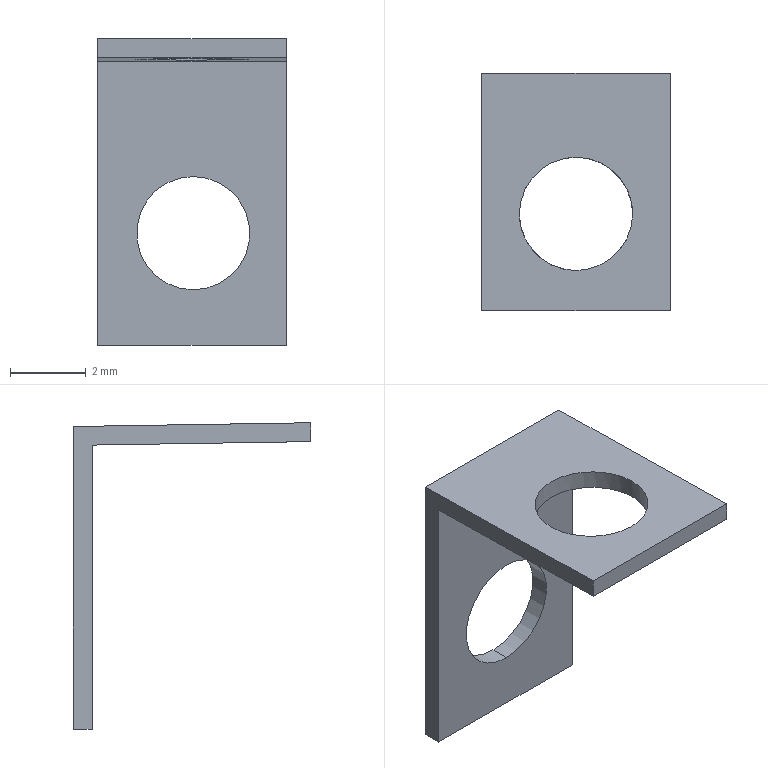Part | SolidWorks | features SplitBody 1 | 1 solid | 12 faces | box 5 x 6.285 x 8.118 mm | volume 27.45 mm3 | plane 8 | cylinder 4 | commonest cylinder face diameters 3 x4
STEP:
#1=CARTESIAN_POINT('',(-22.821,-45.477,-19.331));
#2=VERTEX_POINT('',#1);
#3=CARTESIAN_POINT('',(-19.821,-45.477,-19.331));
#4=VERTEX_POINT('',#3);
#5=CARTESIAN_POINT('',(-22.821,-45.477,-19.331));
#6=CARTESIAN_POINT('',(-22.821,-48.477,-19.284));
#7=CARTESIAN_POINT('',(-19.821,-48.477,-19.284));
#8=CARTESIAN_POINT('',(-19.821,-45.477,-19.331));
#9=(BOUNDED_CURVE()B_SPLINE_CURVE(3,(#5,#6,#7,#8),.UNSPECIFIED.,.F.,.F.)B_SPLINE_CURVE_WITH_KNOTS((4,4),(4.712,7.854),.UNSPECIFIED.)CURVE()GEOMETRIC_REPRESENTATION_ITEM()RATIONAL_B_SPLINE_CURVE((1.,0.3333,0.3333,1.))REPRESENTATION_ITEM(''));
#10=EDGE_CURVE('',#2,#4,#9,.T.);
#11=ORIENTED_EDGE('',*,*,#10,.F.);
#12=CARTESIAN_POINT('',(-22.821,-45.477,-18.831));
#13=VERTEX_POINT('',#12);
#14=CARTESIAN_POINT('',(-22.821,-45.477,-30.));
#15=DIRECTION('',(0.,0.,1.));
#16=VECTOR('',#15,1000.);
#17=LINE('',#14,#16);
#18=EDGE_CURVE('',#2,#13,#17,.T.);
#19=ORIENTED_EDGE('',*,*,#18,.T.);
#20=CARTESIAN_POINT('',(-19.821,-45.477,-18.831));
#21=VERTEX_POINT('',#20);
#22=CARTESIAN_POINT('',(-19.821,-45.477,-18.831));
#23=CARTESIAN_POINT('',(-19.821,-48.477,-18.784));
#24=CARTESIAN_POINT('',(-22.821,-48.477,-18.784));
#25=CARTESIAN_POINT('',(-22.821,-45.477,-18.831));
#26=(BOUNDED_CURVE()B_SPLINE_CURVE(3,(#22,#23,#24,#25),.UNSPECIFIED.,.F.,.F.)B_SPLINE_CURVE_WITH_KNOTS((4,4),(4.712,7.854),.UNSPECIFIED.)CURVE()GEOMETRIC_REPRESENTATION_ITEM()RATIONAL_B_SPLINE_CURVE((1.,0.3333,0.3333,1.))REPRESENTATION_ITEM(''));
#27=EDGE_CURVE('',#21,#13,#26,.T.);
#28=ORIENTED_EDGE('',*,*,#27,.F.);
#29=CARTESIAN_POINT('',(-19.821,-45.477,-30.));
#30=DIRECTION('',(0.,0.,1.));
#31=VECTOR('',#30,1000.);
#32=LINE('',#29,#31);
#33=EDGE_CURVE('',#4,#21,#32,.T.);
#34=ORIENTED_EDGE('',*,*,#33,.F.);
#35=EDGE_LOOP('',(#11,#19,#28,#34));
#36=FACE_OUTER_BOUND('',#35,.T.);
#37=CARTESIAN_POINT('',(-21.321,-45.477,-30.));
#38=DIRECTION('',(0.,0.,1.));
#39=DIRECTION('',(1.,0.,0.));
#40=AXIS2_PLACEMENT_3D('',#37,#38,#39);
#41=CYLINDRICAL_SURFACE('',#40,1.5);
#42=ADVANCED_FACE('',(#36),#41,.F.);
#43=CARTESIAN_POINT('',(-21.288,-41.756,-22.441));
#44=VERTEX_POINT('',#43);
#45=CARTESIAN_POINT('',(-21.288,-41.756,-25.441));
#46=VERTEX_POINT('',#45);
#47=CARTESIAN_POINT('',(-21.288,-41.756,-23.941));
#48=DIRECTION('',(0.,-1.,0.));
#49=DIRECTION('',(0.,0.,-1.));
#50=AXIS2_PLACEMENT_3D('',#47,#48,#49);
#51=CIRCLE('',#50,1.5);
#52=EDGE_CURVE('',#44,#46,#51,.T.);
#53=ORIENTED_EDGE('',*,*,#52,.F.);
#54=CARTESIAN_POINT('',(-21.288,-42.256,-22.441));
#55=VERTEX_POINT('',#54);
#56=CARTESIAN_POINT('',(-21.288,-37.256,-22.441));
#57=DIRECTION('',(0.,-1.,0.));
#58=VECTOR('',#57,1000.);
#59=LINE('',#56,#58);
#60=EDGE_CURVE('',#44,#55,#59,.T.);
#61=ORIENTED_EDGE('',*,*,#60,.T.);
#62=CARTESIAN_POINT('',(-21.288,-42.256,-25.441));
#63=VERTEX_POINT('',#62);
#64=CARTESIAN_POINT('',(-21.288,-42.256,-23.941));
#65=DIRECTION('',(0.,1.,0.));
#66=DIRECTION('',(0.,0.,1.));
#67=AXIS2_PLACEMENT_3D('',#64,#65,#66);
#68=CIRCLE('',#67,1.5);
#69=EDGE_CURVE('',#63,#55,#68,.T.);
#70=ORIENTED_EDGE('',*,*,#69,.F.);
#71=CARTESIAN_POINT('',(-21.288,-37.256,-25.441));
#72=DIRECTION('',(0.,-1.,0.));
#73=VECTOR('',#72,1000.);
#74=LINE('',#71,#73);
#75=EDGE_CURVE('',#46,#63,#74,.T.);
#76=ORIENTED_EDGE('',*,*,#75,.F.);
#77=EDGE_LOOP('',(#53,#61,#70,#76));
#78=FACE_OUTER_BOUND('',#77,.T.);
#79=CARTESIAN_POINT('',(-21.288,-37.256,-23.941));
#80=DIRECTION('',(0.,-1.,0.));
#81=DIRECTION('',(0.,0.,-1.));
#82=AXIS2_PLACEMENT_3D('',#79,#80,#81);
#83=CYLINDRICAL_SURFACE('',#82,1.5);
#84=ADVANCED_FACE('',(#78),#83,.F.);
#85=CARTESIAN_POINT('',(-23.821,-48.041,-18.791));
#86=VERTEX_POINT('',#85);
#87=CARTESIAN_POINT('',(-23.821,-48.041,-19.291));
#88=VERTEX_POINT('',#87);
#89=CARTESIAN_POINT('',(-23.821,-48.041,-18.791));
#90=DIRECTION('',(0.,0.,-1.));
#91=VECTOR('',#90,1000.);
#92=LINE('',#89,#91);
#93=EDGE_CURVE('',#86,#88,#92,.T.);
#94=ORIENTED_EDGE('',*,*,#93,.T.);
#95=CARTESIAN_POINT('',(-18.821,-48.041,-19.291));
#96=VERTEX_POINT('',#95);
#97=CARTESIAN_POINT('',(-18.821,-48.041,-19.291));
#98=DIRECTION('',(-1.,0.,0.));
#99=VECTOR('',#98,1000.);
#100=LINE('',#97,#99);
#101=EDGE_CURVE('',#96,#88,#100,.T.);
#102=ORIENTED_EDGE('',*,*,#101,.F.);
#103=CARTESIAN_POINT('',(-18.821,-48.041,-18.791));
#104=VERTEX_POINT('',#103);
#105=CARTESIAN_POINT('',(-18.821,-48.041,-18.791));
#106=DIRECTION('',(0.,0.,-1.));
#107=VECTOR('',#106,1000.);
#108=LINE('',#105,#107);
#109=EDGE_CURVE('',#104,#96,#108,.T.);
#110=ORIENTED_EDGE('',*,*,#109,.F.);
#111=CARTESIAN_POINT('',(-18.821,-48.041,-18.791));
#112=DIRECTION('',(-1.,0.,0.));
#113=VECTOR('',#112,1000.);
#114=LINE('',#111,#113);
#115=EDGE_CURVE('',#104,#86,#114,.T.);
#116=ORIENTED_EDGE('',*,*,#115,.T.);
#117=EDGE_LOOP('',(#94,#102,#110,#116));
#118=FACE_OUTER_BOUND('',#117,.T.);
#119=CARTESIAN_POINT('',(-18.821,-48.041,-18.791));
#120=DIRECTION('',(0.,1.,0.));
#121=DIRECTION('',(0.,0.,1.));
#122=AXIS2_PLACEMENT_3D('',#119,#120,#121);
#123=PLANE('',#122);
#124=ADVANCED_FACE('',(#118),#123,.F.);
#125=CARTESIAN_POINT('',(-19.821,-45.477,-19.331));
#126=CARTESIAN_POINT('',(-19.821,-42.477,-19.379));
#127=CARTESIAN_POINT('',(-22.821,-42.477,-19.379));
#128=CARTESIAN_POINT('',(-22.821,-45.477,-19.331));
#129=(BOUNDED_CURVE()B_SPLINE_CURVE(3,(#125,#126,#127,#128),.UNSPECIFIED.,.F.,.F.)B_SPLINE_CURVE_WITH_KNOTS((4,4),(1.571,4.712),.UNSPECIFIED.)CURVE()GEOMETRIC_REPRESENTATION_ITEM()RATIONAL_B_SPLINE_CURVE((1.,0.3333,0.3333,1.))REPRESENTATION_ITEM(''));
#130=EDGE_CURVE('',#4,#2,#129,.T.);
#131=ORIENTED_EDGE('',*,*,#130,.T.);
#132=ORIENTED_EDGE('',*,*,#10,.T.);
#133=EDGE_LOOP('',(#131,#132));
#134=FACE_BOUND('',#133,.T.);
#135=CARTESIAN_POINT('',(-23.821,-42.256,-19.382));
#136=VERTEX_POINT('',#135);
#137=CARTESIAN_POINT('',(-23.821,-48.041,-19.291));
#138=DIRECTION('',(0.,0.9999,-0.01579));
#139=VECTOR('',#138,1000.);
#140=LINE('',#137,#139);
#141=EDGE_CURVE('',#88,#136,#140,.T.);
#142=ORIENTED_EDGE('',*,*,#141,.T.);
#143=CARTESIAN_POINT('',(-18.821,-42.256,-19.382));
#144=VERTEX_POINT('',#143);
#145=CARTESIAN_POINT('',(-18.821,-42.256,-19.382));
#146=DIRECTION('',(-1.,0.,0.));
#147=VECTOR('',#146,1000.);
#148=LINE('',#145,#147);
#149=EDGE_CURVE('',#144,#136,#148,.T.);
#150=ORIENTED_EDGE('',*,*,#149,.F.);
#151=CARTESIAN_POINT('',(-18.821,-48.041,-19.291));
#152=DIRECTION('',(0.,0.9999,-0.01579));
#153=VECTOR('',#152,1000.);
#154=LINE('',#151,#153);
#155=EDGE_CURVE('',#96,#144,#154,.T.);
#156=ORIENTED_EDGE('',*,*,#155,.F.);
#157=ORIENTED_EDGE('',*,*,#101,.T.);
#158=EDGE_LOOP('',(#142,#150,#156,#157));
#159=FACE_OUTER_BOUND('',#158,.T.);
#160=CARTESIAN_POINT('',(-18.821,-48.041,-19.291));
#161=DIRECTION('',(0.,0.01579,0.9999));
#162=DIRECTION('',(0.,-0.9999,0.01579));
#163=AXIS2_PLACEMENT_3D('',#160,#161,#162);
#164=PLANE('',#163);
#165=ADVANCED_FACE('',(#134,#159),#164,.F.);
#166=ORIENTED_EDGE('',*,*,#69,.T.);
#167=CARTESIAN_POINT('',(-21.288,-42.256,-23.941));
#168=DIRECTION('',(0.,1.,0.));
#169=DIRECTION('',(0.,0.,1.));
#170=AXIS2_PLACEMENT_3D('',#167,#168,#169);
#171=CIRCLE('',#170,1.5);
#172=EDGE_CURVE('',#55,#63,#171,.T.);
#173=ORIENTED_EDGE('',*,*,#172,.T.);
#174=EDGE_LOOP('',(#166,#173));
#175=FACE_BOUND('',#174,.T.);
#176=CARTESIAN_POINT('',(-23.821,-42.256,-26.909));
#177=VERTEX_POINT('',#176);
#178=CARTESIAN_POINT('',(-23.821,-42.256,-19.382));
#179=DIRECTION('',(0.,0.,-1.));
#180=VECTOR('',#179,1000.);
#181=LINE('',#178,#180);
#182=EDGE_CURVE('',#136,#177,#181,.T.);
#183=ORIENTED_EDGE('',*,*,#182,.T.);
#184=CARTESIAN_POINT('',(-18.821,-42.256,-26.909));
#185=VERTEX_POINT('',#184);
#186=CARTESIAN_POINT('',(-18.821,-42.256,-26.909));
#187=DIRECTION('',(-1.,0.,0.));
#188=VECTOR('',#187,1000.);
#189=LINE('',#186,#188);
#190=EDGE_CURVE('',#185,#177,#189,.T.);
#191=ORIENTED_EDGE('',*,*,#190,.F.);
#192=CARTESIAN_POINT('',(-18.821,-42.256,-19.382));
#193=DIRECTION('',(0.,0.,-1.));
#194=VECTOR('',#193,1000.);
#195=LINE('',#192,#194);
#196=EDGE_CURVE('',#144,#185,#195,.T.);
#197=ORIENTED_EDGE('',*,*,#196,.F.);
#198=ORIENTED_EDGE('',*,*,#149,.T.);
#199=EDGE_LOOP('',(#183,#191,#197,#198));
#200=FACE_OUTER_BOUND('',#199,.T.);
#201=CARTESIAN_POINT('',(-18.821,-42.256,-19.382));
#202=DIRECTION('',(0.,1.,0.));
#203=DIRECTION('',(0.,0.,1.));
#204=AXIS2_PLACEMENT_3D('',#201,#202,#203);
#205=PLANE('',#204);
#206=ADVANCED_FACE('',(#175,#200),#205,.F.);
#207=CARTESIAN_POINT('',(-23.821,-41.756,-26.909));
#208=VERTEX_POINT('',#207);
#209=CARTESIAN_POINT('',(-23.821,-41.756,-26.909));
#210=DIRECTION('',(0.,1.,0.));
#211=VECTOR('',#210,1000.);
#212=LINE('',#209,#211);
#213=EDGE_CURVE('',#177,#208,#212,.T.);
#214=ORIENTED_EDGE('',*,*,#213,.T.);
#215=CARTESIAN_POINT('',(-18.821,-41.756,-26.909));
#216=VERTEX_POINT('',#215);
#217=CARTESIAN_POINT('',(-18.821,-41.756,-26.909));
#218=DIRECTION('',(-1.,0.,0.));
#219=VECTOR('',#218,1000.);
#220=LINE('',#217,#219);
#221=EDGE_CURVE('',#216,#208,#220,.T.);
#222=ORIENTED_EDGE('',*,*,#221,.F.);
#223=CARTESIAN_POINT('',(-18.821,-41.756,-26.909));
#224=DIRECTION('',(0.,1.,0.));
#225=VECTOR('',#224,1000.);
#226=LINE('',#223,#225);
#227=EDGE_CURVE('',#185,#216,#226,.T.);
#228=ORIENTED_EDGE('',*,*,#227,.F.);
#229=ORIENTED_EDGE('',*,*,#190,.T.);
#230=EDGE_LOOP('',(#214,#222,#228,#229));
#231=FACE_OUTER_BOUND('',#230,.T.);
#232=CARTESIAN_POINT('',(-18.821,-41.756,-26.909));
#233=DIRECTION('',(0.,0.,1.));
#234=DIRECTION('',(1.,0.,0.));
#235=AXIS2_PLACEMENT_3D('',#232,#233,#234);
#236=PLANE('',#235);
#237=ADVANCED_FACE('',(#231),#236,.F.);
#238=CARTESIAN_POINT('',(-21.288,-41.756,-23.941));
#239=DIRECTION('',(0.,-1.,0.));
#240=DIRECTION('',(0.,0.,-1.));
#241=AXIS2_PLACEMENT_3D('',#238,#239,#240);
#242=CIRCLE('',#241,1.5);
#243=EDGE_CURVE('',#46,#44,#242,.T.);
#244=ORIENTED_EDGE('',*,*,#243,.T.);
#245=ORIENTED_EDGE('',*,*,#52,.T.);
#246=EDGE_LOOP('',(#244,#245));
#247=FACE_BOUND('',#246,.T.);
#248=CARTESIAN_POINT('',(-23.821,-41.756,-18.89));
#249=VERTEX_POINT('',#248);
#250=CARTESIAN_POINT('',(-23.821,-41.756,-18.89));
#251=DIRECTION('',(0.,0.,1.));
#252=VECTOR('',#251,1000.);
#253=LINE('',#250,#252);
#254=EDGE_CURVE('',#208,#249,#253,.T.);
#255=ORIENTED_EDGE('',*,*,#254,.T.);
#256=CARTESIAN_POINT('',(-18.821,-41.756,-18.89));
#257=VERTEX_POINT('',#256);
#258=CARTESIAN_POINT('',(-18.821,-41.756,-18.89));
#259=DIRECTION('',(-1.,0.,0.));
#260=VECTOR('',#259,1000.);
#261=LINE('',#258,#260);
#262=EDGE_CURVE('',#257,#249,#261,.T.);
#263=ORIENTED_EDGE('',*,*,#262,.F.);
#264=CARTESIAN_POINT('',(-18.821,-41.756,-18.89));
#265=DIRECTION('',(0.,0.,1.));
#266=VECTOR('',#265,1000.);
#267=LINE('',#264,#266);
#268=EDGE_CURVE('',#216,#257,#267,.T.);
#269=ORIENTED_EDGE('',*,*,#268,.F.);
#270=ORIENTED_EDGE('',*,*,#221,.T.);
#271=EDGE_LOOP('',(#255,#263,#269,#270));
#272=FACE_OUTER_BOUND('',#271,.T.);
#273=CARTESIAN_POINT('',(-18.821,-41.756,-18.89));
#274=DIRECTION('',(0.,-1.,0.));
#275=DIRECTION('',(0.,0.,-1.));
#276=AXIS2_PLACEMENT_3D('',#273,#274,#275);
#277=PLANE('',#276);
#278=ADVANCED_FACE('',(#247,#272),#277,.F.);
#279=ORIENTED_EDGE('',*,*,#27,.T.);
#280=CARTESIAN_POINT('',(-22.821,-45.477,-18.831));
#281=CARTESIAN_POINT('',(-22.821,-42.477,-18.879));
#282=CARTESIAN_POINT('',(-19.821,-42.477,-18.879));
#283=CARTESIAN_POINT('',(-19.821,-45.477,-18.831));
#284=(BOUNDED_CURVE()B_SPLINE_CURVE(3,(#280,#281,#282,#283),.UNSPECIFIED.,.F.,.F.)B_SPLINE_CURVE_WITH_KNOTS((4,4),(1.571,4.712),.UNSPECIFIED.)CURVE()GEOMETRIC_REPRESENTATION_ITEM()RATIONAL_B_SPLINE_CURVE((1.,0.3333,0.3333,1.))REPRESENTATION_ITEM(''));
#285=EDGE_CURVE('',#13,#21,#284,.T.);
#286=ORIENTED_EDGE('',*,*,#285,.T.);
#287=EDGE_LOOP('',(#279,#286));
#288=FACE_BOUND('',#287,.T.);
#289=CARTESIAN_POINT('',(-23.821,-48.041,-18.791));
#290=DIRECTION('',(0.,-0.9999,0.01579));
#291=VECTOR('',#290,1000.);
#292=LINE('',#289,#291);
#293=EDGE_CURVE('',#249,#86,#292,.T.);
#294=ORIENTED_EDGE('',*,*,#293,.T.);
#295=ORIENTED_EDGE('',*,*,#115,.F.);
#296=CARTESIAN_POINT('',(-18.821,-48.041,-18.791));
#297=DIRECTION('',(0.,-0.9999,0.01579));
#298=VECTOR('',#297,1000.);
#299=LINE('',#296,#298);
#300=EDGE_CURVE('',#257,#104,#299,.T.);
#301=ORIENTED_EDGE('',*,*,#300,.F.);
#302=ORIENTED_EDGE('',*,*,#262,.T.);
#303=EDGE_LOOP('',(#294,#295,#301,#302));
#304=FACE_OUTER_BOUND('',#303,.T.);
#305=CARTESIAN_POINT('',(-18.821,-48.041,-18.791));
#306=DIRECTION('',(0.,-0.01579,-0.9999));
#307=DIRECTION('',(0.,0.9999,-0.01579));
#308=AXIS2_PLACEMENT_3D('',#305,#306,#307);
#309=PLANE('',#308);
#310=ADVANCED_FACE('',(#288,#304),#309,.F.);
#311=ORIENTED_EDGE('',*,*,#109,.T.);
#312=ORIENTED_EDGE('',*,*,#155,.T.);
#313=ORIENTED_EDGE('',*,*,#196,.T.);
#314=ORIENTED_EDGE('',*,*,#227,.T.);
#315=ORIENTED_EDGE('',*,*,#268,.T.);
#316=ORIENTED_EDGE('',*,*,#300,.T.);
#317=EDGE_LOOP('',(#311,#312,#313,#314,#315,#316));
#318=FACE_OUTER_BOUND('',#317,.T.);
#319=CARTESIAN_POINT('',(-18.821,0.,0.));
#320=DIRECTION('',(-1.,0.,0.));
#321=DIRECTION('',(0.,0.,1.));
#322=AXIS2_PLACEMENT_3D('',#319,#320,#321);
#323=PLANE('',#322);
#324=ADVANCED_FACE('',(#318),#323,.F.);
#325=ORIENTED_EDGE('',*,*,#93,.F.);
#326=ORIENTED_EDGE('',*,*,#293,.F.);
#327=ORIENTED_EDGE('',*,*,#254,.F.);
#328=ORIENTED_EDGE('',*,*,#213,.F.);
#329=ORIENTED_EDGE('',*,*,#182,.F.);
#330=ORIENTED_EDGE('',*,*,#141,.F.);
#331=EDGE_LOOP('',(#325,#326,#327,#328,#329,#330));
#332=FACE_OUTER_BOUND('',#331,.T.);
#333=CARTESIAN_POINT('',(-23.821,0.,0.));
#334=DIRECTION('',(-1.,0.,0.));
#335=DIRECTION('',(0.,0.,1.));
#336=AXIS2_PLACEMENT_3D('',#333,#334,#335);
#337=PLANE('',#336);
#338=ADVANCED_FACE('',(#332),#337,.T.);
#339=ORIENTED_EDGE('',*,*,#60,.F.);
#340=ORIENTED_EDGE('',*,*,#243,.F.);
#341=ORIENTED_EDGE('',*,*,#75,.T.);
#342=ORIENTED_EDGE('',*,*,#172,.F.);
#343=EDGE_LOOP('',(#339,#340,#341,#342));
#344=FACE_OUTER_BOUND('',#343,.T.);
#345=CARTESIAN_POINT('',(-21.288,-37.256,-23.941));
#346=DIRECTION('',(0.,-1.,0.));
#347=DIRECTION('',(0.,0.,-1.));
#348=AXIS2_PLACEMENT_3D('',#345,#346,#347);
#349=CYLINDRICAL_SURFACE('',#348,1.5);
#350=ADVANCED_FACE('',(#344),#349,.F.);
#351=ORIENTED_EDGE('',*,*,#18,.F.);
#352=ORIENTED_EDGE('',*,*,#130,.F.);
#353=ORIENTED_EDGE('',*,*,#33,.T.);
#354=ORIENTED_EDGE('',*,*,#285,.F.);
#355=EDGE_LOOP('',(#351,#352,#353,#354));
#356=FACE_OUTER_BOUND('',#355,.T.);
#357=CARTESIAN_POINT('',(-21.321,-45.477,-30.));
#358=DIRECTION('',(0.,0.,1.));
#359=DIRECTION('',(1.,0.,0.));
#360=AXIS2_PLACEMENT_3D('',#357,#358,#359);
#361=CYLINDRICAL_SURFACE('',#360,1.5);
#362=ADVANCED_FACE('',(#356),#361,.F.);
#363=CLOSED_SHELL('',(#42,#84,#124,#165,#206,#237,#278,#310,#324,#338,#350,#362));
#364=MANIFOLD_SOLID_BREP('',#363);
#365=CARTESIAN_POINT('',(0.,0.,0.));
#366=DIRECTION('',(0.,0.,1.));
#367=DIRECTION('',(1.,0.,0.));
#368=AXIS2_PLACEMENT_3D('',#365,#366,#367);
#369=(LENGTH_UNIT()NAMED_UNIT(*)SI_UNIT(.MILLI.,.METRE.));
#370=UNCERTAINTY_MEASURE_WITH_UNIT(LENGTH_MEASURE(0.00001),#369,'','');
#371=(NAMED_UNIT(*)PLANE_ANGLE_UNIT()SI_UNIT($,.RADIAN.));
#372=(NAMED_UNIT(*)SI_UNIT($,.STERADIAN.)SOLID_ANGLE_UNIT());
#373=(GEOMETRIC_REPRESENTATION_CONTEXT(3)GLOBAL_UNCERTAINTY_ASSIGNED_CONTEXT((#370))GLOBAL_UNIT_ASSIGNED_CONTEXT((#369,#371,#372))REPRESENTATION_CONTEXT('',''));
#374=ADVANCED_BREP_SHAPE_REPRESENTATION('',(#364,#368),#373);